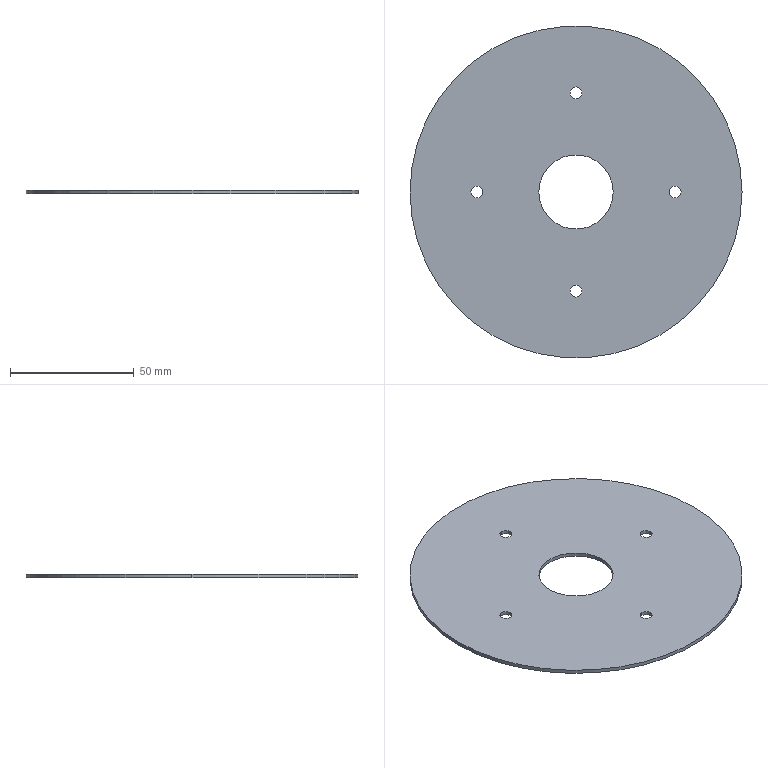Part | SolidWorks | features BaseBody 1 | 1 solid | 14 faces | box 134 x 134 x 1.5 mm | volume 19985 mm3 | cylinder 12 | plane 2 | commonest cylinder face diameters 4.8 x8 30 x2 134 x2
STEP:
#1=CARTESIAN_POINT('',(0.,42.4,-1.5));
#2=VERTEX_POINT('',#1);
#3=CARTESIAN_POINT('',(0.,42.4,0.));
#4=VERTEX_POINT('',#3);
#5=CARTESIAN_POINT('',(0.,42.4,0.));
#6=DIRECTION('',(0.,0.,1.));
#7=VECTOR('',#6,1000.);
#8=LINE('',#5,#7);
#9=EDGE_CURVE('',#2,#4,#8,.T.);
#10=ORIENTED_EDGE('',*,*,#9,.F.);
#11=CARTESIAN_POINT('',(0.,37.6,-1.5));
#12=VERTEX_POINT('',#11);
#13=CARTESIAN_POINT('',(0.,40.,-1.5));
#14=DIRECTION('',(0.,0.,1.));
#15=DIRECTION('',(0.,-1.,0.));
#16=AXIS2_PLACEMENT_3D('',#13,#14,#15);
#17=CIRCLE('',#16,2.4);
#18=EDGE_CURVE('',#12,#2,#17,.T.);
#19=ORIENTED_EDGE('',*,*,#18,.F.);
#20=CARTESIAN_POINT('',(0.,37.6,0.));
#21=VERTEX_POINT('',#20);
#22=CARTESIAN_POINT('',(0.,37.6,0.));
#23=DIRECTION('',(0.,0.,1.));
#24=VECTOR('',#23,1000.);
#25=LINE('',#22,#24);
#26=EDGE_CURVE('',#12,#21,#25,.T.);
#27=ORIENTED_EDGE('',*,*,#26,.T.);
#28=CARTESIAN_POINT('',(0.,40.,0.));
#29=DIRECTION('',(0.,0.,1.));
#30=DIRECTION('',(0.,-1.,0.));
#31=AXIS2_PLACEMENT_3D('',#28,#29,#30);
#32=CIRCLE('',#31,2.4);
#33=EDGE_CURVE('',#21,#4,#32,.T.);
#34=ORIENTED_EDGE('',*,*,#33,.T.);
#35=EDGE_LOOP('',(#10,#19,#27,#34));
#36=FACE_OUTER_BOUND('',#35,.T.);
#37=CARTESIAN_POINT('',(0.,40.,0.));
#38=DIRECTION('',(0.,0.,1.));
#39=DIRECTION('',(0.,-1.,0.));
#40=AXIS2_PLACEMENT_3D('',#37,#38,#39);
#41=CYLINDRICAL_SURFACE('',#40,2.4);
#42=ADVANCED_FACE('',(#36),#41,.F.);
#43=CARTESIAN_POINT('',(42.4,0.,-1.5));
#44=VERTEX_POINT('',#43);
#45=CARTESIAN_POINT('',(42.4,0.,0.));
#46=VERTEX_POINT('',#45);
#47=CARTESIAN_POINT('',(42.4,0.,0.));
#48=DIRECTION('',(0.,0.,1.));
#49=VECTOR('',#48,1000.);
#50=LINE('',#47,#49);
#51=EDGE_CURVE('',#44,#46,#50,.T.);
#52=ORIENTED_EDGE('',*,*,#51,.F.);
#53=CARTESIAN_POINT('',(37.6,0.,-1.5));
#54=VERTEX_POINT('',#53);
#55=CARTESIAN_POINT('',(40.,0.,-1.5));
#56=DIRECTION('',(0.,0.,1.));
#57=DIRECTION('',(-1.,0.,0.));
#58=AXIS2_PLACEMENT_3D('',#55,#56,#57);
#59=CIRCLE('',#58,2.4);
#60=EDGE_CURVE('',#54,#44,#59,.T.);
#61=ORIENTED_EDGE('',*,*,#60,.F.);
#62=CARTESIAN_POINT('',(37.6,0.,0.));
#63=VERTEX_POINT('',#62);
#64=CARTESIAN_POINT('',(37.6,0.,0.));
#65=DIRECTION('',(0.,0.,1.));
#66=VECTOR('',#65,1000.);
#67=LINE('',#64,#66);
#68=EDGE_CURVE('',#54,#63,#67,.T.);
#69=ORIENTED_EDGE('',*,*,#68,.T.);
#70=CARTESIAN_POINT('',(40.,0.,0.));
#71=DIRECTION('',(0.,0.,1.));
#72=DIRECTION('',(-1.,0.,0.));
#73=AXIS2_PLACEMENT_3D('',#70,#71,#72);
#74=CIRCLE('',#73,2.4);
#75=EDGE_CURVE('',#63,#46,#74,.T.);
#76=ORIENTED_EDGE('',*,*,#75,.T.);
#77=EDGE_LOOP('',(#52,#61,#69,#76));
#78=FACE_OUTER_BOUND('',#77,.T.);
#79=CARTESIAN_POINT('',(40.,0.,0.));
#80=DIRECTION('',(0.,0.,1.));
#81=DIRECTION('',(-1.,0.,0.));
#82=AXIS2_PLACEMENT_3D('',#79,#80,#81);
#83=CYLINDRICAL_SURFACE('',#82,2.4);
#84=ADVANCED_FACE('',(#78),#83,.F.);
#85=CARTESIAN_POINT('',(0.,-42.4,-1.5));
#86=VERTEX_POINT('',#85);
#87=CARTESIAN_POINT('',(0.,-42.4,0.));
#88=VERTEX_POINT('',#87);
#89=CARTESIAN_POINT('',(0.,-42.4,0.));
#90=DIRECTION('',(0.,0.,1.));
#91=VECTOR('',#90,1000.);
#92=LINE('',#89,#91);
#93=EDGE_CURVE('',#86,#88,#92,.T.);
#94=ORIENTED_EDGE('',*,*,#93,.F.);
#95=CARTESIAN_POINT('',(0.,-37.6,-1.5));
#96=VERTEX_POINT('',#95);
#97=CARTESIAN_POINT('',(0.,-40.,-1.5));
#98=DIRECTION('',(0.,0.,1.));
#99=DIRECTION('',(0.,1.,0.));
#100=AXIS2_PLACEMENT_3D('',#97,#98,#99);
#101=CIRCLE('',#100,2.4);
#102=EDGE_CURVE('',#96,#86,#101,.T.);
#103=ORIENTED_EDGE('',*,*,#102,.F.);
#104=CARTESIAN_POINT('',(0.,-37.6,0.));
#105=VERTEX_POINT('',#104);
#106=CARTESIAN_POINT('',(0.,-37.6,0.));
#107=DIRECTION('',(0.,0.,1.));
#108=VECTOR('',#107,1000.);
#109=LINE('',#106,#108);
#110=EDGE_CURVE('',#96,#105,#109,.T.);
#111=ORIENTED_EDGE('',*,*,#110,.T.);
#112=CARTESIAN_POINT('',(0.,-40.,0.));
#113=DIRECTION('',(0.,0.,1.));
#114=DIRECTION('',(0.,1.,0.));
#115=AXIS2_PLACEMENT_3D('',#112,#113,#114);
#116=CIRCLE('',#115,2.4);
#117=EDGE_CURVE('',#105,#88,#116,.T.);
#118=ORIENTED_EDGE('',*,*,#117,.T.);
#119=EDGE_LOOP('',(#94,#103,#111,#118));
#120=FACE_OUTER_BOUND('',#119,.T.);
#121=CARTESIAN_POINT('',(0.,-40.,0.));
#122=DIRECTION('',(0.,0.,1.));
#123=DIRECTION('',(0.,1.,0.));
#124=AXIS2_PLACEMENT_3D('',#121,#122,#123);
#125=CYLINDRICAL_SURFACE('',#124,2.4);
#126=ADVANCED_FACE('',(#120),#125,.F.);
#127=CARTESIAN_POINT('',(-42.4,0.,-1.5));
#128=VERTEX_POINT('',#127);
#129=CARTESIAN_POINT('',(-42.4,0.,0.));
#130=VERTEX_POINT('',#129);
#131=CARTESIAN_POINT('',(-42.4,0.,0.));
#132=DIRECTION('',(0.,0.,1.));
#133=VECTOR('',#132,1000.);
#134=LINE('',#131,#133);
#135=EDGE_CURVE('',#128,#130,#134,.T.);
#136=ORIENTED_EDGE('',*,*,#135,.F.);
#137=CARTESIAN_POINT('',(-37.6,0.,-1.5));
#138=VERTEX_POINT('',#137);
#139=CARTESIAN_POINT('',(-40.,0.,-1.5));
#140=DIRECTION('',(0.,0.,1.));
#141=DIRECTION('',(1.,0.,0.));
#142=AXIS2_PLACEMENT_3D('',#139,#140,#141);
#143=CIRCLE('',#142,2.4);
#144=EDGE_CURVE('',#138,#128,#143,.T.);
#145=ORIENTED_EDGE('',*,*,#144,.F.);
#146=CARTESIAN_POINT('',(-37.6,0.,0.));
#147=VERTEX_POINT('',#146);
#148=CARTESIAN_POINT('',(-37.6,0.,0.));
#149=DIRECTION('',(0.,0.,1.));
#150=VECTOR('',#149,1000.);
#151=LINE('',#148,#150);
#152=EDGE_CURVE('',#138,#147,#151,.T.);
#153=ORIENTED_EDGE('',*,*,#152,.T.);
#154=CARTESIAN_POINT('',(-40.,0.,0.));
#155=DIRECTION('',(0.,0.,1.));
#156=DIRECTION('',(1.,0.,0.));
#157=AXIS2_PLACEMENT_3D('',#154,#155,#156);
#158=CIRCLE('',#157,2.4);
#159=EDGE_CURVE('',#147,#130,#158,.T.);
#160=ORIENTED_EDGE('',*,*,#159,.T.);
#161=EDGE_LOOP('',(#136,#145,#153,#160));
#162=FACE_OUTER_BOUND('',#161,.T.);
#163=CARTESIAN_POINT('',(-40.,0.,0.));
#164=DIRECTION('',(0.,0.,1.));
#165=DIRECTION('',(1.,0.,0.));
#166=AXIS2_PLACEMENT_3D('',#163,#164,#165);
#167=CYLINDRICAL_SURFACE('',#166,2.4);
#168=ADVANCED_FACE('',(#162),#167,.F.);
#169=CARTESIAN_POINT('',(-15.,0.,-1.5));
#170=VERTEX_POINT('',#169);
#171=CARTESIAN_POINT('',(-15.,0.,0.));
#172=VERTEX_POINT('',#171);
#173=CARTESIAN_POINT('',(-15.,0.,-1.5));
#174=DIRECTION('',(0.,0.,1.));
#175=VECTOR('',#174,1000.);
#176=LINE('',#173,#175);
#177=EDGE_CURVE('',#170,#172,#176,.T.);
#178=ORIENTED_EDGE('',*,*,#177,.F.);
#179=CARTESIAN_POINT('',(15.,0.,-1.5));
#180=VERTEX_POINT('',#179);
#181=CARTESIAN_POINT('',(0.,0.,-1.5));
#182=DIRECTION('',(0.,0.,1.));
#183=DIRECTION('',(1.,0.,0.));
#184=AXIS2_PLACEMENT_3D('',#181,#182,#183);
#185=CIRCLE('',#184,15.);
#186=EDGE_CURVE('',#180,#170,#185,.T.);
#187=ORIENTED_EDGE('',*,*,#186,.F.);
#188=CARTESIAN_POINT('',(15.,0.,0.));
#189=VERTEX_POINT('',#188);
#190=CARTESIAN_POINT('',(15.,0.,-1.5));
#191=DIRECTION('',(0.,0.,1.));
#192=VECTOR('',#191,1000.);
#193=LINE('',#190,#192);
#194=EDGE_CURVE('',#180,#189,#193,.T.);
#195=ORIENTED_EDGE('',*,*,#194,.T.);
#196=CARTESIAN_POINT('',(0.,0.,0.));
#197=DIRECTION('',(0.,0.,1.));
#198=DIRECTION('',(1.,0.,0.));
#199=AXIS2_PLACEMENT_3D('',#196,#197,#198);
#200=CIRCLE('',#199,15.);
#201=EDGE_CURVE('',#189,#172,#200,.T.);
#202=ORIENTED_EDGE('',*,*,#201,.T.);
#203=EDGE_LOOP('',(#178,#187,#195,#202));
#204=FACE_OUTER_BOUND('',#203,.T.);
#205=CARTESIAN_POINT('',(0.,0.,-1.5));
#206=DIRECTION('',(0.,0.,1.));
#207=DIRECTION('',(1.,0.,0.));
#208=AXIS2_PLACEMENT_3D('',#205,#206,#207);
#209=CYLINDRICAL_SURFACE('',#208,15.);
#210=ADVANCED_FACE('',(#204),#209,.F.);
#211=ORIENTED_EDGE('',*,*,#201,.F.);
#212=CARTESIAN_POINT('',(0.,0.,0.));
#213=DIRECTION('',(0.,0.,1.));
#214=DIRECTION('',(1.,0.,0.));
#215=AXIS2_PLACEMENT_3D('',#212,#213,#214);
#216=CIRCLE('',#215,15.);
#217=EDGE_CURVE('',#172,#189,#216,.T.);
#218=ORIENTED_EDGE('',*,*,#217,.F.);
#219=EDGE_LOOP('',(#211,#218));
#220=FACE_BOUND('',#219,.T.);
#221=ORIENTED_EDGE('',*,*,#159,.F.);
#222=CARTESIAN_POINT('',(-40.,0.,0.));
#223=DIRECTION('',(0.,0.,1.));
#224=DIRECTION('',(1.,0.,0.));
#225=AXIS2_PLACEMENT_3D('',#222,#223,#224);
#226=CIRCLE('',#225,2.4);
#227=EDGE_CURVE('',#130,#147,#226,.T.);
#228=ORIENTED_EDGE('',*,*,#227,.F.);
#229=EDGE_LOOP('',(#221,#228));
#230=FACE_BOUND('',#229,.T.);
#231=ORIENTED_EDGE('',*,*,#117,.F.);
#232=CARTESIAN_POINT('',(0.,-40.,0.));
#233=DIRECTION('',(0.,0.,1.));
#234=DIRECTION('',(0.,1.,0.));
#235=AXIS2_PLACEMENT_3D('',#232,#233,#234);
#236=CIRCLE('',#235,2.4);
#237=EDGE_CURVE('',#88,#105,#236,.T.);
#238=ORIENTED_EDGE('',*,*,#237,.F.);
#239=EDGE_LOOP('',(#231,#238));
#240=FACE_BOUND('',#239,.T.);
#241=ORIENTED_EDGE('',*,*,#75,.F.);
#242=CARTESIAN_POINT('',(40.,0.,0.));
#243=DIRECTION('',(0.,0.,1.));
#244=DIRECTION('',(-1.,0.,0.));
#245=AXIS2_PLACEMENT_3D('',#242,#243,#244);
#246=CIRCLE('',#245,2.4);
#247=EDGE_CURVE('',#46,#63,#246,.T.);
#248=ORIENTED_EDGE('',*,*,#247,.F.);
#249=EDGE_LOOP('',(#241,#248));
#250=FACE_BOUND('',#249,.T.);
#251=ORIENTED_EDGE('',*,*,#33,.F.);
#252=CARTESIAN_POINT('',(0.,40.,0.));
#253=DIRECTION('',(0.,0.,1.));
#254=DIRECTION('',(0.,-1.,0.));
#255=AXIS2_PLACEMENT_3D('',#252,#253,#254);
#256=CIRCLE('',#255,2.4);
#257=EDGE_CURVE('',#4,#21,#256,.T.);
#258=ORIENTED_EDGE('',*,*,#257,.F.);
#259=EDGE_LOOP('',(#251,#258));
#260=FACE_BOUND('',#259,.T.);
#261=CARTESIAN_POINT('',(67.,0.,0.));
#262=VERTEX_POINT('',#261);
#263=CARTESIAN_POINT('',(-67.,0.,0.));
#264=VERTEX_POINT('',#263);
#265=CARTESIAN_POINT('',(0.,0.,0.));
#266=DIRECTION('',(0.,0.,1.));
#267=DIRECTION('',(1.,0.,0.));
#268=AXIS2_PLACEMENT_3D('',#265,#266,#267);
#269=CIRCLE('',#268,67.);
#270=EDGE_CURVE('',#262,#264,#269,.T.);
#271=ORIENTED_EDGE('',*,*,#270,.T.);
#272=CARTESIAN_POINT('',(0.,0.,0.));
#273=DIRECTION('',(0.,0.,1.));
#274=DIRECTION('',(1.,0.,0.));
#275=AXIS2_PLACEMENT_3D('',#272,#273,#274);
#276=CIRCLE('',#275,67.);
#277=EDGE_CURVE('',#264,#262,#276,.T.);
#278=ORIENTED_EDGE('',*,*,#277,.T.);
#279=EDGE_LOOP('',(#271,#278));
#280=FACE_OUTER_BOUND('',#279,.T.);
#281=CARTESIAN_POINT('',(0.,0.,0.));
#282=DIRECTION('',(0.,0.,1.));
#283=DIRECTION('',(1.,0.,0.));
#284=AXIS2_PLACEMENT_3D('',#281,#282,#283);
#285=PLANE('',#284);
#286=ADVANCED_FACE('',(#220,#230,#240,#250,#260,#280),#285,.T.);
#287=ORIENTED_EDGE('',*,*,#186,.T.);
#288=CARTESIAN_POINT('',(0.,0.,-1.5));
#289=DIRECTION('',(0.,0.,1.));
#290=DIRECTION('',(1.,0.,0.));
#291=AXIS2_PLACEMENT_3D('',#288,#289,#290);
#292=CIRCLE('',#291,15.);
#293=EDGE_CURVE('',#170,#180,#292,.T.);
#294=ORIENTED_EDGE('',*,*,#293,.T.);
#295=EDGE_LOOP('',(#287,#294));
#296=FACE_BOUND('',#295,.T.);
#297=ORIENTED_EDGE('',*,*,#144,.T.);
#298=CARTESIAN_POINT('',(-40.,0.,-1.5));
#299=DIRECTION('',(0.,0.,1.));
#300=DIRECTION('',(1.,0.,0.));
#301=AXIS2_PLACEMENT_3D('',#298,#299,#300);
#302=CIRCLE('',#301,2.4);
#303=EDGE_CURVE('',#128,#138,#302,.T.);
#304=ORIENTED_EDGE('',*,*,#303,.T.);
#305=EDGE_LOOP('',(#297,#304));
#306=FACE_BOUND('',#305,.T.);
#307=ORIENTED_EDGE('',*,*,#102,.T.);
#308=CARTESIAN_POINT('',(0.,-40.,-1.5));
#309=DIRECTION('',(0.,0.,1.));
#310=DIRECTION('',(0.,1.,0.));
#311=AXIS2_PLACEMENT_3D('',#308,#309,#310);
#312=CIRCLE('',#311,2.4);
#313=EDGE_CURVE('',#86,#96,#312,.T.);
#314=ORIENTED_EDGE('',*,*,#313,.T.);
#315=EDGE_LOOP('',(#307,#314));
#316=FACE_BOUND('',#315,.T.);
#317=ORIENTED_EDGE('',*,*,#60,.T.);
#318=CARTESIAN_POINT('',(40.,0.,-1.5));
#319=DIRECTION('',(0.,0.,1.));
#320=DIRECTION('',(-1.,0.,0.));
#321=AXIS2_PLACEMENT_3D('',#318,#319,#320);
#322=CIRCLE('',#321,2.4);
#323=EDGE_CURVE('',#44,#54,#322,.T.);
#324=ORIENTED_EDGE('',*,*,#323,.T.);
#325=EDGE_LOOP('',(#317,#324));
#326=FACE_BOUND('',#325,.T.);
#327=ORIENTED_EDGE('',*,*,#18,.T.);
#328=CARTESIAN_POINT('',(0.,40.,-1.5));
#329=DIRECTION('',(0.,0.,1.));
#330=DIRECTION('',(0.,-1.,0.));
#331=AXIS2_PLACEMENT_3D('',#328,#329,#330);
#332=CIRCLE('',#331,2.4);
#333=EDGE_CURVE('',#2,#12,#332,.T.);
#334=ORIENTED_EDGE('',*,*,#333,.T.);
#335=EDGE_LOOP('',(#327,#334));
#336=FACE_BOUND('',#335,.T.);
#337=CARTESIAN_POINT('',(67.,0.,-1.5));
#338=VERTEX_POINT('',#337);
#339=CARTESIAN_POINT('',(-67.,0.,-1.5));
#340=VERTEX_POINT('',#339);
#341=CARTESIAN_POINT('',(0.,0.,-1.5));
#342=DIRECTION('',(0.,0.,1.));
#343=DIRECTION('',(1.,0.,0.));
#344=AXIS2_PLACEMENT_3D('',#341,#342,#343);
#345=CIRCLE('',#344,67.);
#346=EDGE_CURVE('',#338,#340,#345,.T.);
#347=ORIENTED_EDGE('',*,*,#346,.F.);
#348=CARTESIAN_POINT('',(0.,0.,-1.5));
#349=DIRECTION('',(0.,0.,1.));
#350=DIRECTION('',(1.,0.,0.));
#351=AXIS2_PLACEMENT_3D('',#348,#349,#350);
#352=CIRCLE('',#351,67.);
#353=EDGE_CURVE('',#340,#338,#352,.T.);
#354=ORIENTED_EDGE('',*,*,#353,.F.);
#355=EDGE_LOOP('',(#347,#354));
#356=FACE_OUTER_BOUND('',#355,.T.);
#357=CARTESIAN_POINT('',(0.,0.,-1.5));
#358=DIRECTION('',(0.,0.,1.));
#359=DIRECTION('',(1.,0.,0.));
#360=AXIS2_PLACEMENT_3D('',#357,#358,#359);
#361=PLANE('',#360);
#362=ADVANCED_FACE('',(#296,#306,#316,#326,#336,#356),#361,.F.);
#363=CARTESIAN_POINT('',(-67.,0.,-1.5));
#364=DIRECTION('',(0.,0.,1.));
#365=VECTOR('',#364,1000.);
#366=LINE('',#363,#365);
#367=EDGE_CURVE('',#340,#264,#366,.T.);
#368=ORIENTED_EDGE('',*,*,#367,.F.);
#369=ORIENTED_EDGE('',*,*,#353,.T.);
#370=CARTESIAN_POINT('',(67.,0.,-1.5));
#371=DIRECTION('',(0.,0.,1.));
#372=VECTOR('',#371,1000.);
#373=LINE('',#370,#372);
#374=EDGE_CURVE('',#338,#262,#373,.T.);
#375=ORIENTED_EDGE('',*,*,#374,.T.);
#376=ORIENTED_EDGE('',*,*,#277,.F.);
#377=EDGE_LOOP('',(#368,#369,#375,#376));
#378=FACE_OUTER_BOUND('',#377,.T.);
#379=CARTESIAN_POINT('',(0.,0.,-1.5));
#380=DIRECTION('',(0.,0.,1.));
#381=DIRECTION('',(1.,0.,0.));
#382=AXIS2_PLACEMENT_3D('',#379,#380,#381);
#383=CYLINDRICAL_SURFACE('',#382,67.);
#384=ADVANCED_FACE('',(#378),#383,.T.);
#385=ORIENTED_EDGE('',*,*,#346,.T.);
#386=ORIENTED_EDGE('',*,*,#367,.T.);
#387=ORIENTED_EDGE('',*,*,#270,.F.);
#388=ORIENTED_EDGE('',*,*,#374,.F.);
#389=EDGE_LOOP('',(#385,#386,#387,#388));
#390=FACE_OUTER_BOUND('',#389,.T.);
#391=CARTESIAN_POINT('',(0.,0.,-1.5));
#392=DIRECTION('',(0.,0.,1.));
#393=DIRECTION('',(1.,0.,0.));
#394=AXIS2_PLACEMENT_3D('',#391,#392,#393);
#395=CYLINDRICAL_SURFACE('',#394,67.);
#396=ADVANCED_FACE('',(#390),#395,.T.);
#397=ORIENTED_EDGE('',*,*,#293,.F.);
#398=ORIENTED_EDGE('',*,*,#177,.T.);
#399=ORIENTED_EDGE('',*,*,#217,.T.);
#400=ORIENTED_EDGE('',*,*,#194,.F.);
#401=EDGE_LOOP('',(#397,#398,#399,#400));
#402=FACE_OUTER_BOUND('',#401,.T.);
#403=CARTESIAN_POINT('',(0.,0.,-1.5));
#404=DIRECTION('',(0.,0.,1.));
#405=DIRECTION('',(1.,0.,0.));
#406=AXIS2_PLACEMENT_3D('',#403,#404,#405);
#407=CYLINDRICAL_SURFACE('',#406,15.);
#408=ADVANCED_FACE('',(#402),#407,.F.);
#409=ORIENTED_EDGE('',*,*,#303,.F.);
#410=ORIENTED_EDGE('',*,*,#135,.T.);
#411=ORIENTED_EDGE('',*,*,#227,.T.);
#412=ORIENTED_EDGE('',*,*,#152,.F.);
#413=EDGE_LOOP('',(#409,#410,#411,#412));
#414=FACE_OUTER_BOUND('',#413,.T.);
#415=CARTESIAN_POINT('',(-40.,0.,0.));
#416=DIRECTION('',(0.,0.,1.));
#417=DIRECTION('',(1.,0.,0.));
#418=AXIS2_PLACEMENT_3D('',#415,#416,#417);
#419=CYLINDRICAL_SURFACE('',#418,2.4);
#420=ADVANCED_FACE('',(#414),#419,.F.);
#421=ORIENTED_EDGE('',*,*,#313,.F.);
#422=ORIENTED_EDGE('',*,*,#93,.T.);
#423=ORIENTED_EDGE('',*,*,#237,.T.);
#424=ORIENTED_EDGE('',*,*,#110,.F.);
#425=EDGE_LOOP('',(#421,#422,#423,#424));
#426=FACE_OUTER_BOUND('',#425,.T.);
#427=CARTESIAN_POINT('',(0.,-40.,0.));
#428=DIRECTION('',(0.,0.,1.));
#429=DIRECTION('',(0.,1.,0.));
#430=AXIS2_PLACEMENT_3D('',#427,#428,#429);
#431=CYLINDRICAL_SURFACE('',#430,2.4);
#432=ADVANCED_FACE('',(#426),#431,.F.);
#433=ORIENTED_EDGE('',*,*,#323,.F.);
#434=ORIENTED_EDGE('',*,*,#51,.T.);
#435=ORIENTED_EDGE('',*,*,#247,.T.);
#436=ORIENTED_EDGE('',*,*,#68,.F.);
#437=EDGE_LOOP('',(#433,#434,#435,#436));
#438=FACE_OUTER_BOUND('',#437,.T.);
#439=CARTESIAN_POINT('',(40.,0.,0.));
#440=DIRECTION('',(0.,0.,1.));
#441=DIRECTION('',(-1.,0.,0.));
#442=AXIS2_PLACEMENT_3D('',#439,#440,#441);
#443=CYLINDRICAL_SURFACE('',#442,2.4);
#444=ADVANCED_FACE('',(#438),#443,.F.);
#445=ORIENTED_EDGE('',*,*,#333,.F.);
#446=ORIENTED_EDGE('',*,*,#9,.T.);
#447=ORIENTED_EDGE('',*,*,#257,.T.);
#448=ORIENTED_EDGE('',*,*,#26,.F.);
#449=EDGE_LOOP('',(#445,#446,#447,#448));
#450=FACE_OUTER_BOUND('',#449,.T.);
#451=CARTESIAN_POINT('',(0.,40.,0.));
#452=DIRECTION('',(0.,0.,1.));
#453=DIRECTION('',(0.,-1.,0.));
#454=AXIS2_PLACEMENT_3D('',#451,#452,#453);
#455=CYLINDRICAL_SURFACE('',#454,2.4);
#456=ADVANCED_FACE('',(#450),#455,.F.);
#457=CLOSED_SHELL('',(#42,#84,#126,#168,#210,#286,#362,#384,#396,#408,#420,#432,#444,#456));
#458=MANIFOLD_SOLID_BREP('',#457);
#459=CARTESIAN_POINT('',(0.,0.,0.));
#460=DIRECTION('',(0.,0.,1.));
#461=DIRECTION('',(1.,0.,0.));
#462=AXIS2_PLACEMENT_3D('',#459,#460,#461);
#463=(LENGTH_UNIT()NAMED_UNIT(*)SI_UNIT(.MILLI.,.METRE.));
#464=UNCERTAINTY_MEASURE_WITH_UNIT(LENGTH_MEASURE(0.00001),#463,'','');
#465=(NAMED_UNIT(*)PLANE_ANGLE_UNIT()SI_UNIT($,.RADIAN.));
#466=(NAMED_UNIT(*)SI_UNIT($,.STERADIAN.)SOLID_ANGLE_UNIT());
#467=(GEOMETRIC_REPRESENTATION_CONTEXT(3)GLOBAL_UNCERTAINTY_ASSIGNED_CONTEXT((#464))GLOBAL_UNIT_ASSIGNED_CONTEXT((#463,#465,#466))REPRESENTATION_CONTEXT('',''));
#468=ADVANCED_BREP_SHAPE_REPRESENTATION('',(#458,#462),#467);